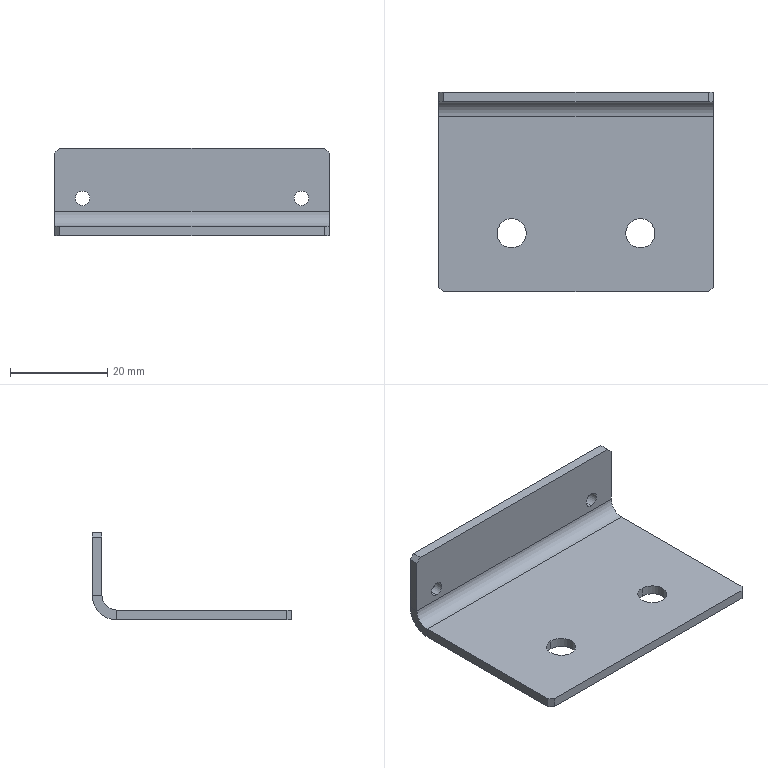Part | STEP file | 227H056396 BKT_Default | 1 solid | 26 faces | box 56.5 x 41.063 x 18 mm | volume 6109 mm3 | plane 16 | cylinder 10 | commonest cylinder face diameters 6 x5 3 x4 10 x1